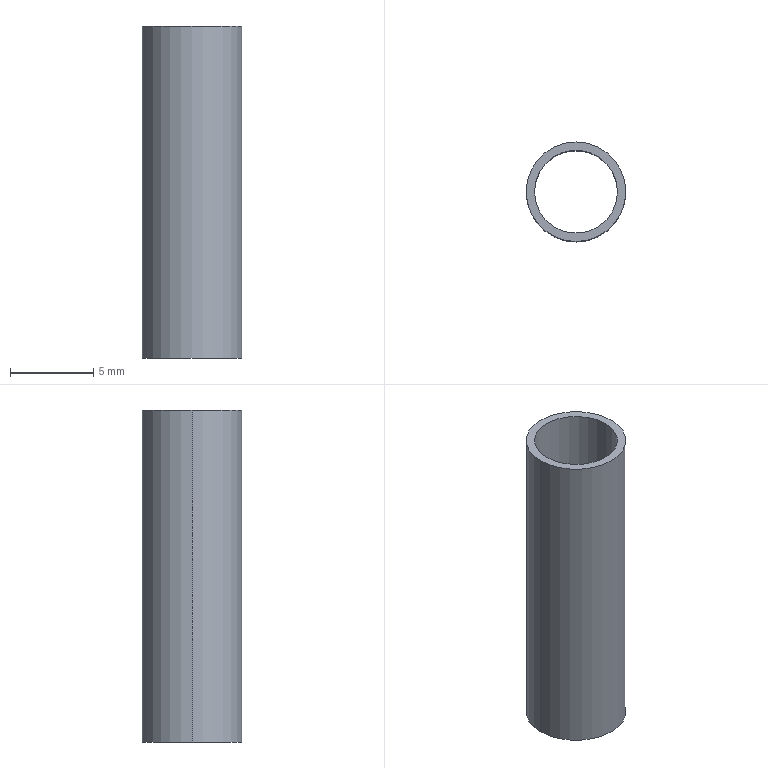Part | STEP file | 102000006988 | 1 solid | 6 faces | box 6 x 6 x 20 mm | volume 172.788 mm3 | cylinder 4 | plane 2 | commonest cylinder face diameters 5 x2 6 x2
STEP:
#1=CARTESIAN_POINT('',(-2.5,0.,20.));
#2=VERTEX_POINT('',#1);
#3=CARTESIAN_POINT('',(2.5,0.,20.));
#4=VERTEX_POINT('',#3);
#5=CARTESIAN_POINT('',(0.,0.,20.));
#6=DIRECTION('',(0.,0.,-1.));
#7=AXIS2_PLACEMENT_3D('',#5,#6,$);
#8=CIRCLE('',#7,2.5);
#9=EDGE_CURVE('',#2,#4,#8,.F.);
#10=ORIENTED_EDGE('',*,*,#9,.T.);
#11=CARTESIAN_POINT('',(2.5,0.,0.));
#12=VERTEX_POINT('',#11);
#13=CARTESIAN_POINT('',(2.5,0.,20.));
#14=DIRECTION('',(0.,0.,-1.));
#15=VECTOR('',#14,1.);
#16=LINE('',#13,#15);
#17=EDGE_CURVE('',#4,#12,#16,.T.);
#18=ORIENTED_EDGE('',*,*,#17,.T.);
#19=CARTESIAN_POINT('',(-2.5,0.,0.));
#20=VERTEX_POINT('',#19);
#21=CARTESIAN_POINT('',(0.,0.,0.));
#22=DIRECTION('',(0.,0.,-1.));
#23=AXIS2_PLACEMENT_3D('',#21,#22,$);
#24=CIRCLE('',#23,2.5);
#25=EDGE_CURVE('',#20,#12,#24,.F.);
#26=ORIENTED_EDGE('',*,*,#25,.F.);
#27=CARTESIAN_POINT('',(-2.5,0.,20.));
#28=DIRECTION('',(0.,0.,-1.));
#29=VECTOR('',#28,1.);
#30=LINE('',#27,#29);
#31=EDGE_CURVE('',#2,#20,#30,.T.);
#32=ORIENTED_EDGE('',*,*,#31,.F.);
#33=EDGE_LOOP('',(#10,#18,#26,#32));
#34=FACE_OUTER_BOUND('',#33,.T.);
#35=CARTESIAN_POINT('',(0.,0.,20.));
#36=DIRECTION('',(0.,0.,-1.));
#37=DIRECTION('',(1.,0.,0.));
#38=AXIS2_PLACEMENT_3D('',#35,#36,#37);
#39=CYLINDRICAL_SURFACE('',#38,2.5);
#40=ADVANCED_FACE('',(#34),#39,.F.);
#41=CARTESIAN_POINT('',(-3.,0.,20.));
#42=VERTEX_POINT('',#41);
#43=CARTESIAN_POINT('',(3.,0.,20.));
#44=VERTEX_POINT('',#43);
#45=CARTESIAN_POINT('',(0.,0.,20.));
#46=DIRECTION('',(0.,0.,1.));
#47=AXIS2_PLACEMENT_3D('',#45,#46,$);
#48=CIRCLE('',#47,3.);
#49=EDGE_CURVE('',#42,#44,#48,.T.);
#50=ORIENTED_EDGE('',*,*,#49,.T.);
#51=CARTESIAN_POINT('',(0.,0.,20.));
#52=DIRECTION('',(0.,0.,1.));
#53=AXIS2_PLACEMENT_3D('',#51,#52,$);
#54=CIRCLE('',#53,3.);
#55=EDGE_CURVE('',#44,#42,#54,.T.);
#56=ORIENTED_EDGE('',*,*,#55,.T.);
#57=EDGE_LOOP('',(#50,#56));
#58=FACE_OUTER_BOUND('',#57,.T.);
#59=ORIENTED_EDGE('',*,*,#9,.F.);
#60=CARTESIAN_POINT('',(0.,0.,20.));
#61=DIRECTION('',(0.,0.,1.));
#62=AXIS2_PLACEMENT_3D('',#60,#61,$);
#63=CIRCLE('',#62,2.5);
#64=EDGE_CURVE('',#4,#2,#63,.T.);
#65=ORIENTED_EDGE('',*,*,#64,.F.);
#66=EDGE_LOOP('',(#59,#65));
#67=FACE_BOUND('',#66,.T.);
#68=CARTESIAN_POINT('',(0.,0.,20.));
#69=DIRECTION('',(0.,0.,1.));
#70=DIRECTION('',(1.,0.,0.));
#71=AXIS2_PLACEMENT_3D('',#68,#69,#70);
#72=PLANE('',#71);
#73=ADVANCED_FACE('',(#58,#67),#72,.T.);
#74=ORIENTED_EDGE('',*,*,#17,.F.);
#75=ORIENTED_EDGE('',*,*,#64,.T.);
#76=ORIENTED_EDGE('',*,*,#31,.T.);
#77=CARTESIAN_POINT('',(0.,0.,0.));
#78=DIRECTION('',(0.,0.,-1.));
#79=AXIS2_PLACEMENT_3D('',#77,#78,$);
#80=CIRCLE('',#79,2.5);
#81=EDGE_CURVE('',#12,#20,#80,.F.);
#82=ORIENTED_EDGE('',*,*,#81,.F.);
#83=EDGE_LOOP('',(#74,#75,#76,#82));
#84=FACE_OUTER_BOUND('',#83,.T.);
#85=CARTESIAN_POINT('',(0.,0.,20.));
#86=DIRECTION('',(0.,0.,-1.));
#87=DIRECTION('',(-1.,0.,0.));
#88=AXIS2_PLACEMENT_3D('',#85,#86,#87);
#89=CYLINDRICAL_SURFACE('',#88,2.5);
#90=ADVANCED_FACE('',(#84),#89,.F.);
#91=CARTESIAN_POINT('',(-3.,0.,0.));
#92=VERTEX_POINT('',#91);
#93=CARTESIAN_POINT('',(3.,0.,0.));
#94=VERTEX_POINT('',#93);
#95=CARTESIAN_POINT('',(0.,0.,0.));
#96=DIRECTION('',(0.,0.,1.));
#97=AXIS2_PLACEMENT_3D('',#95,#96,$);
#98=CIRCLE('',#97,3.);
#99=EDGE_CURVE('',#92,#94,#98,.T.);
#100=ORIENTED_EDGE('',*,*,#99,.F.);
#101=CARTESIAN_POINT('',(0.,0.,0.));
#102=DIRECTION('',(0.,0.,1.));
#103=AXIS2_PLACEMENT_3D('',#101,#102,$);
#104=CIRCLE('',#103,3.);
#105=EDGE_CURVE('',#94,#92,#104,.T.);
#106=ORIENTED_EDGE('',*,*,#105,.F.);
#107=EDGE_LOOP('',(#100,#106));
#108=FACE_OUTER_BOUND('',#107,.T.);
#109=ORIENTED_EDGE('',*,*,#25,.T.);
#110=ORIENTED_EDGE('',*,*,#81,.T.);
#111=EDGE_LOOP('',(#109,#110));
#112=FACE_BOUND('',#111,.T.);
#113=CARTESIAN_POINT('',(0.,0.,0.));
#114=DIRECTION('',(0.,0.,1.));
#115=DIRECTION('',(1.,0.,0.));
#116=AXIS2_PLACEMENT_3D('',#113,#114,#115);
#117=PLANE('',#116);
#118=ADVANCED_FACE('',(#108,#112),#117,.F.);
#119=CARTESIAN_POINT('',(3.,0.,20.));
#120=DIRECTION('',(0.,0.,-1.));
#121=VECTOR('',#120,1.);
#122=LINE('',#119,#121);
#123=EDGE_CURVE('',#44,#94,#122,.T.);
#124=ORIENTED_EDGE('',*,*,#123,.F.);
#125=ORIENTED_EDGE('',*,*,#49,.F.);
#126=CARTESIAN_POINT('',(-3.,0.,20.));
#127=DIRECTION('',(0.,0.,-1.));
#128=VECTOR('',#127,1.);
#129=LINE('',#126,#128);
#130=EDGE_CURVE('',#42,#92,#129,.T.);
#131=ORIENTED_EDGE('',*,*,#130,.T.);
#132=ORIENTED_EDGE('',*,*,#99,.T.);
#133=EDGE_LOOP('',(#124,#125,#131,#132));
#134=FACE_OUTER_BOUND('',#133,.T.);
#135=CARTESIAN_POINT('',(0.,0.,20.));
#136=DIRECTION('',(0.,0.,-1.));
#137=DIRECTION('',(1.,0.,0.));
#138=AXIS2_PLACEMENT_3D('',#135,#136,#137);
#139=CYLINDRICAL_SURFACE('',#138,3.);
#140=ADVANCED_FACE('',(#134),#139,.T.);
#141=ORIENTED_EDGE('',*,*,#55,.F.);
#142=ORIENTED_EDGE('',*,*,#123,.T.);
#143=ORIENTED_EDGE('',*,*,#105,.T.);
#144=ORIENTED_EDGE('',*,*,#130,.F.);
#145=EDGE_LOOP('',(#141,#142,#143,#144));
#146=FACE_OUTER_BOUND('',#145,.T.);
#147=CARTESIAN_POINT('',(0.,0.,20.));
#148=DIRECTION('',(0.,0.,-1.));
#149=DIRECTION('',(-1.,0.,0.));
#150=AXIS2_PLACEMENT_3D('',#147,#148,#149);
#151=CYLINDRICAL_SURFACE('',#150,3.);
#152=ADVANCED_FACE('',(#146),#151,.T.);
#153=CLOSED_SHELL('',(#40,#73,#90,#118,#140,#152));
#154=MANIFOLD_SOLID_BREP('',#153);
#155=(LENGTH_UNIT()NAMED_UNIT(*)SI_UNIT(.MILLI.,.METRE.));
#156=UNCERTAINTY_MEASURE_WITH_UNIT(LENGTH_MEASURE(0.005),#155,'','');
#157=(NAMED_UNIT(*)PLANE_ANGLE_UNIT()SI_UNIT($,.RADIAN.));
#158=(NAMED_UNIT(*)SI_UNIT($,.STERADIAN.)SOLID_ANGLE_UNIT());
#159=(GEOMETRIC_REPRESENTATION_CONTEXT(3)GLOBAL_UNCERTAINTY_ASSIGNED_CONTEXT((#156))GLOBAL_UNIT_ASSIGNED_CONTEXT((#155,#157,#158))REPRESENTATION_CONTEXT('',''));
#160=ADVANCED_BREP_SHAPE_REPRESENTATION('',(#154),#159);